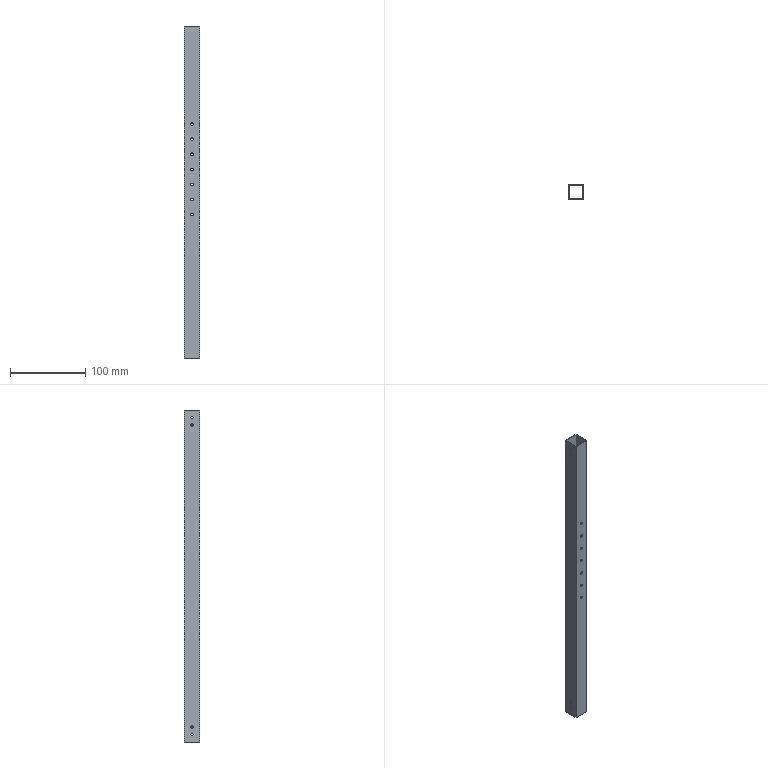Part | SolidWorks | features BaseBody 1 | 1 solid | 54 faces | box 20 x 20 x 440 mm | volume 33241 mm3 | cylinder 44 | plane 10 | commonest cylinder face diameters 3.5 x28 3.2 x16